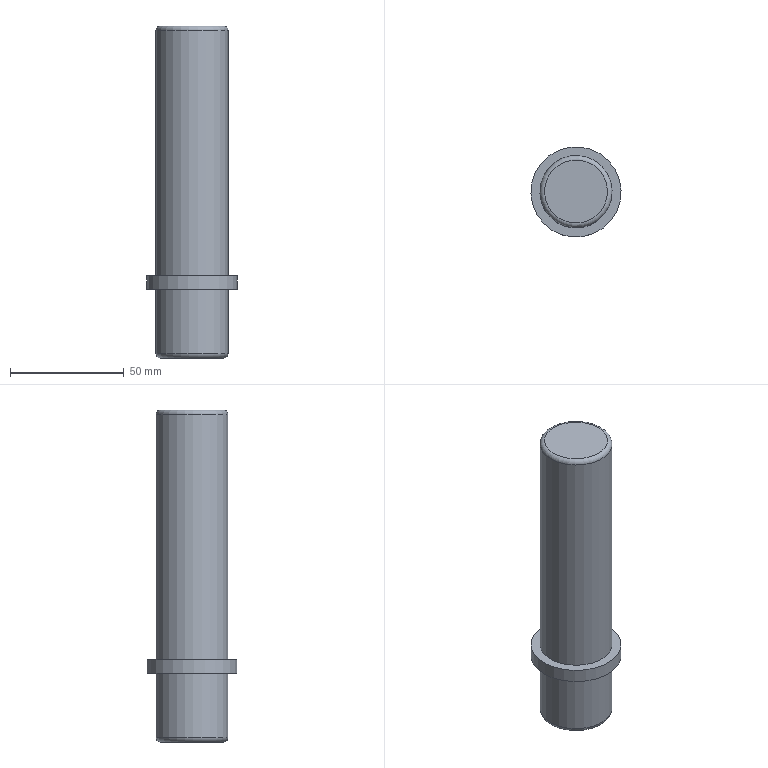Part | STEP file | 1_id1374_x_t | 1 solid | 13 faces | box 39.688 x 39.688 x 146.05 mm | volume 117725 mm3 | plane 5 | cylinder 4 | cone 2 | torus 2 | commonest cylinder face diameters 31.75 x2 4.2 x1 39.688 x1
STEP:
#1=CARTESIAN_POINT('',(0.,0.,0.));
#2=DIRECTION('',(0.,0.,1.));
#3=DIRECTION('',(1.,0.,0.));
#4=AXIS2_PLACEMENT_3D('',#1,#2,#3);
#5=CARTESIAN_POINT('',(862.606,287.316,48.075));
#6=VERTEX_POINT('',#5);
#7=CARTESIAN_POINT('',(862.925,287.5,48.075));
#8=DIRECTION('',(0.,0.,1.));
#9=DIRECTION('',(-0.866,-0.5,0.));
#10=AXIS2_PLACEMENT_3D('',#7,#8,#9);
#11=CIRCLE('',#10,0.3679);
#12=CARTESIAN_POINT('',(862.925,287.5,48.075));
#13=DIRECTION('',(0.,0.,1.));
#14=DIRECTION('',(-0.5,0.866,0.));
#15=AXIS2_PLACEMENT_3D('',#12,#13,#14);
#16=PLANE('',#15);
#17=CARTESIAN_POINT('',(0.0001996,0.));
#18=DIRECTION('',(0.,1.));
#19=AXIS2_PLACEMENT_2D('',#17,#18);
#20=CIRCLE('',#19,0.3679);
#21=(GEOMETRIC_REPRESENTATION_CONTEXT(2)PARAMETRIC_REPRESENTATION_CONTEXT()REPRESENTATION_CONTEXT('',''));
#22=DEFINITIONAL_REPRESENTATION('',(#20),#21);
#23=PCURVE('',#16,#22);
#24=CARTESIAN_POINT('',(862.925,287.5,47.575));
#25=DIRECTION('',(0.,0.,-1.));
#26=DIRECTION('',(-0.866,-0.5,0.));
#27=AXIS2_PLACEMENT_3D('',#24,#25,#26);
#28=CONICAL_SURFACE('',#27,1.234,1.047);
#29=CARTESIAN_POINT('',(6.283,-0.5));
#30=DIRECTION('',(-1.,0.));
#31=VECTOR('',#30,1.);
#32=LINE('',#29,#31);
#33=(GEOMETRIC_REPRESENTATION_CONTEXT(2)PARAMETRIC_REPRESENTATION_CONTEXT()REPRESENTATION_CONTEXT('',''));
#34=DEFINITIONAL_REPRESENTATION('',(#32),#33);
#35=PCURVE('',#28,#34);
#36=SURFACE_CURVE('',#11,(#23,#35),.PCURVE_S1.);
#37=EDGE_CURVE('',#6,#6,#36,.T.);
#38=ORIENTED_EDGE('',*,*,#37,.F.);
#39=EDGE_LOOP('',(#38));
#40=FACE_BOUND('',#39,.T.);
#41=ADVANCED_FACE('',(#40),#16,.F.);
#42=CARTESIAN_POINT('',(861.106,286.45,47.075));
#43=VERTEX_POINT('',#42);
#44=CARTESIAN_POINT('',(864.744,288.55,47.075));
#45=VERTEX_POINT('',#44);
#46=CARTESIAN_POINT('',(862.925,287.5,47.075));
#47=DIRECTION('',(0.,0.,-1.));
#48=DIRECTION('',(0.866,0.5,0.));
#49=AXIS2_PLACEMENT_3D('',#46,#47,#48);
#50=CIRCLE('',#49,2.1);
#51=CARTESIAN_POINT('',(-3.142,0.5));
#52=DIRECTION('',(1.,0.));
#53=VECTOR('',#52,1.);
#54=LINE('',#51,#53);
#55=(GEOMETRIC_REPRESENTATION_CONTEXT(2)PARAMETRIC_REPRESENTATION_CONTEXT()REPRESENTATION_CONTEXT('',''));
#56=DEFINITIONAL_REPRESENTATION('',(#54),#55);
#57=PCURVE('',#28,#56);
#58=CARTESIAN_POINT('',(862.925,287.5,47.075));
#59=DIRECTION('',(0.,0.,1.));
#60=DIRECTION('',(-0.866,-0.5,0.));
#61=AXIS2_PLACEMENT_3D('',#58,#59,#60);
#62=CYLINDRICAL_SURFACE('',#61,2.1);
#63=CARTESIAN_POINT('',(9.425,0.));
#64=DIRECTION('',(-1.,0.));
#65=VECTOR('',#64,1.);
#66=LINE('',#63,#65);
#67=(GEOMETRIC_REPRESENTATION_CONTEXT(2)PARAMETRIC_REPRESENTATION_CONTEXT()REPRESENTATION_CONTEXT('',''));
#68=DEFINITIONAL_REPRESENTATION('',(#66),#67);
#69=PCURVE('',#62,#68);
#70=SURFACE_CURVE('',#50,(#57,#69),.PCURVE_S1.);
#71=EDGE_CURVE('',#43,#45,#70,.T.);
#72=ORIENTED_EDGE('',*,*,#71,.F.);
#73=CARTESIAN_POINT('',(862.606,287.316,48.075));
#74=CARTESIAN_POINT('',(861.106,286.45,47.075));
#75=B_SPLINE_CURVE_WITH_KNOTS('',1,(#73,#74),.UNSPECIFIED.,.F.,.F.,(2,2),(-1.,1.),.PIECEWISE_BEZIER_KNOTS.);
#76=CARTESIAN_POINT('',(0.,0.));
#77=DIRECTION('',(0.,1.));
#78=VECTOR('',#77,1.);
#79=LINE('',#76,#78);
#80=(GEOMETRIC_REPRESENTATION_CONTEXT(2)PARAMETRIC_REPRESENTATION_CONTEXT()REPRESENTATION_CONTEXT('',''));
#81=DEFINITIONAL_REPRESENTATION('',(#79),#80);
#82=PCURVE('',#28,#81);
#83=CARTESIAN_POINT('',(6.283,0.));
#84=DIRECTION('',(0.,1.));
#85=VECTOR('',#84,1.);
#86=LINE('',#83,#85);
#87=(GEOMETRIC_REPRESENTATION_CONTEXT(2)PARAMETRIC_REPRESENTATION_CONTEXT()REPRESENTATION_CONTEXT('',''));
#88=DEFINITIONAL_REPRESENTATION('',(#86),#87);
#89=PCURVE('',#28,#88);
#90=SEAM_CURVE('',#75,(#82,#89),.PCURVE_S1.);
#91=EDGE_CURVE('',#6,#43,#90,.T.);
#92=ORIENTED_EDGE('',*,*,#91,.F.);
#93=ORIENTED_EDGE('',*,*,#37,.F.);
#94=ORIENTED_EDGE('',*,*,#91,.T.);
#95=CARTESIAN_POINT('',(862.925,287.5,47.075));
#96=DIRECTION('',(0.,0.,-1.));
#97=DIRECTION('',(0.866,0.5,0.));
#98=AXIS2_PLACEMENT_3D('',#95,#96,#97);
#99=CIRCLE('',#98,2.1);
#100=CARTESIAN_POINT('',(3.142,0.5));
#101=DIRECTION('',(1.,0.));
#102=VECTOR('',#101,1.);
#103=LINE('',#100,#102);
#104=(GEOMETRIC_REPRESENTATION_CONTEXT(2)PARAMETRIC_REPRESENTATION_CONTEXT()REPRESENTATION_CONTEXT('',''));
#105=DEFINITIONAL_REPRESENTATION('',(#103),#104);
#106=PCURVE('',#28,#105);
#107=CARTESIAN_POINT('',(9.425,0.));
#108=DIRECTION('',(-1.,0.));
#109=VECTOR('',#108,1.);
#110=LINE('',#107,#109);
#111=(GEOMETRIC_REPRESENTATION_CONTEXT(2)PARAMETRIC_REPRESENTATION_CONTEXT()REPRESENTATION_CONTEXT('',''));
#112=DEFINITIONAL_REPRESENTATION('',(#110),#111);
#113=PCURVE('',#62,#112);
#114=SURFACE_CURVE('',#99,(#106,#113),.PCURVE_S1.);
#115=EDGE_CURVE('',#45,#43,#114,.T.);
#116=ORIENTED_EDGE('',*,*,#115,.F.);
#117=EDGE_LOOP('',(#72,#92,#93,#94,#116));
#118=FACE_BOUND('',#117,.F.);
#119=ADVANCED_FACE('',(#118),#28,.F.);
#120=ORIENTED_EDGE('',*,*,#71,.T.);
#121=CARTESIAN_POINT('',(864.744,288.55,18.575));
#122=VERTEX_POINT('',#121);
#123=CARTESIAN_POINT('',(864.744,288.55,18.575));
#124=CARTESIAN_POINT('',(864.744,288.55,47.075));
#125=B_SPLINE_CURVE_WITH_KNOTS('',1,(#123,#124),.UNSPECIFIED.,.F.,.F.,(2,2),(-28.5,0.),.PIECEWISE_BEZIER_KNOTS.);
#126=CARTESIAN_POINT('',(3.142,0.));
#127=DIRECTION('',(0.,1.));
#128=VECTOR('',#127,1.);
#129=LINE('',#126,#128);
#130=(GEOMETRIC_REPRESENTATION_CONTEXT(2)PARAMETRIC_REPRESENTATION_CONTEXT()REPRESENTATION_CONTEXT('',''));
#131=DEFINITIONAL_REPRESENTATION('',(#129),#130);
#132=PCURVE('',#62,#131);
#133=CARTESIAN_POINT('',(9.425,0.));
#134=DIRECTION('',(0.,1.));
#135=VECTOR('',#134,1.);
#136=LINE('',#133,#135);
#137=(GEOMETRIC_REPRESENTATION_CONTEXT(2)PARAMETRIC_REPRESENTATION_CONTEXT()REPRESENTATION_CONTEXT('',''));
#138=DEFINITIONAL_REPRESENTATION('',(#136),#137);
#139=PCURVE('',#62,#138);
#140=SEAM_CURVE('',#125,(#132,#139),.PCURVE_S1.);
#141=EDGE_CURVE('',#122,#45,#140,.T.);
#142=ORIENTED_EDGE('',*,*,#141,.F.);
#143=CARTESIAN_POINT('',(861.106,286.45,18.575));
#144=VERTEX_POINT('',#143);
#145=CARTESIAN_POINT('',(862.925,287.5,18.575));
#146=DIRECTION('',(0.,0.,1.));
#147=DIRECTION('',(0.866,0.5,0.));
#148=AXIS2_PLACEMENT_3D('',#145,#146,#147);
#149=CIRCLE('',#148,2.1);
#150=CARTESIAN_POINT('',(3.142,-28.5));
#151=DIRECTION('',(1.,0.));
#152=VECTOR('',#151,1.);
#153=LINE('',#150,#152);
#154=(GEOMETRIC_REPRESENTATION_CONTEXT(2)PARAMETRIC_REPRESENTATION_CONTEXT()REPRESENTATION_CONTEXT('',''));
#155=DEFINITIONAL_REPRESENTATION('',(#153),#154);
#156=PCURVE('',#62,#155);
#157=CARTESIAN_POINT('',(862.925,287.5,18.244));
#158=DIRECTION('',(0.,0.,-1.));
#159=DIRECTION('',(-0.866,-0.5,0.));
#160=AXIS2_PLACEMENT_3D('',#157,#158,#159);
#161=CONICAL_SURFACE('',#160,2.431,0.7854);
#162=CARTESIAN_POINT('',(3.142,-0.3313));
#163=DIRECTION('',(-1.,0.));
#164=VECTOR('',#163,1.);
#165=LINE('',#162,#164);
#166=(GEOMETRIC_REPRESENTATION_CONTEXT(2)PARAMETRIC_REPRESENTATION_CONTEXT()REPRESENTATION_CONTEXT('',''));
#167=DEFINITIONAL_REPRESENTATION('',(#165),#166);
#168=PCURVE('',#161,#167);
#169=SURFACE_CURVE('',#149,(#156,#168),.PCURVE_S1.);
#170=EDGE_CURVE('',#122,#144,#169,.T.);
#171=ORIENTED_EDGE('',*,*,#170,.T.);
#172=CARTESIAN_POINT('',(862.925,287.5,18.575));
#173=DIRECTION('',(0.,0.,1.));
#174=DIRECTION('',(0.866,0.5,0.));
#175=AXIS2_PLACEMENT_3D('',#172,#173,#174);
#176=CIRCLE('',#175,2.1);
#177=CARTESIAN_POINT('',(3.142,-28.5));
#178=DIRECTION('',(1.,0.));
#179=VECTOR('',#178,1.);
#180=LINE('',#177,#179);
#181=(GEOMETRIC_REPRESENTATION_CONTEXT(2)PARAMETRIC_REPRESENTATION_CONTEXT()REPRESENTATION_CONTEXT('',''));
#182=DEFINITIONAL_REPRESENTATION('',(#180),#181);
#183=PCURVE('',#62,#182);
#184=CARTESIAN_POINT('',(9.425,-0.3313));
#185=DIRECTION('',(-1.,0.));
#186=VECTOR('',#185,1.);
#187=LINE('',#184,#186);
#188=(GEOMETRIC_REPRESENTATION_CONTEXT(2)PARAMETRIC_REPRESENTATION_CONTEXT()REPRESENTATION_CONTEXT('',''));
#189=DEFINITIONAL_REPRESENTATION('',(#187),#188);
#190=PCURVE('',#161,#189);
#191=SURFACE_CURVE('',#176,(#183,#190),.PCURVE_S1.);
#192=EDGE_CURVE('',#144,#122,#191,.T.);
#193=ORIENTED_EDGE('',*,*,#192,.T.);
#194=ORIENTED_EDGE('',*,*,#141,.T.);
#195=ORIENTED_EDGE('',*,*,#115,.T.);
#196=EDGE_LOOP('',(#120,#142,#171,#193,#194,#195));
#197=FACE_BOUND('',#196,.F.);
#198=ADVANCED_FACE('',(#197),#62,.F.);
#199=CARTESIAN_POINT('',(860.533,286.119,17.912));
#200=VERTEX_POINT('',#199);
#201=CARTESIAN_POINT('',(862.925,287.5,17.912));
#202=DIRECTION('',(0.,0.,1.));
#203=DIRECTION('',(-0.866,-0.5,0.));
#204=AXIS2_PLACEMENT_3D('',#201,#202,#203);
#205=CIRCLE('',#204,2.763);
#206=CARTESIAN_POINT('',(6.283,0.3313));
#207=DIRECTION('',(-1.,0.));
#208=VECTOR('',#207,1.);
#209=LINE('',#206,#208);
#210=(GEOMETRIC_REPRESENTATION_CONTEXT(2)PARAMETRIC_REPRESENTATION_CONTEXT()REPRESENTATION_CONTEXT('',''));
#211=DEFINITIONAL_REPRESENTATION('',(#209),#210);
#212=PCURVE('',#161,#211);
#213=CARTESIAN_POINT('',(862.925,287.5,17.912));
#214=DIRECTION('',(0.,0.,1.));
#215=DIRECTION('',(-0.866,-0.5,0.));
#216=AXIS2_PLACEMENT_3D('',#213,#214,#215);
#217=PLANE('',#216);
#218=CARTESIAN_POINT('',(0.,0.));
#219=DIRECTION('',(1.,0.));
#220=AXIS2_PLACEMENT_2D('',#218,#219);
#221=CIRCLE('',#220,2.763);
#222=(GEOMETRIC_REPRESENTATION_CONTEXT(2)PARAMETRIC_REPRESENTATION_CONTEXT()REPRESENTATION_CONTEXT('',''));
#223=DEFINITIONAL_REPRESENTATION('',(#221),#222);
#224=PCURVE('',#217,#223);
#225=SURFACE_CURVE('',#205,(#212,#224),.PCURVE_S1.);
#226=EDGE_CURVE('',#200,#200,#225,.T.);
#227=ORIENTED_EDGE('',*,*,#226,.T.);
#228=CARTESIAN_POINT('',(861.106,286.45,18.575));
#229=CARTESIAN_POINT('',(860.533,286.119,17.912));
#230=B_SPLINE_CURVE_WITH_KNOTS('',1,(#228,#229),.UNSPECIFIED.,.F.,.F.,(2,2),(-0.4685,0.4685),.PIECEWISE_BEZIER_KNOTS.);
#231=CARTESIAN_POINT('',(0.,0.));
#232=DIRECTION('',(0.,1.));
#233=VECTOR('',#232,1.);
#234=LINE('',#231,#233);
#235=(GEOMETRIC_REPRESENTATION_CONTEXT(2)PARAMETRIC_REPRESENTATION_CONTEXT()REPRESENTATION_CONTEXT('',''));
#236=DEFINITIONAL_REPRESENTATION('',(#234),#235);
#237=PCURVE('',#161,#236);
#238=CARTESIAN_POINT('',(6.283,0.));
#239=DIRECTION('',(0.,1.));
#240=VECTOR('',#239,1.);
#241=LINE('',#238,#240);
#242=(GEOMETRIC_REPRESENTATION_CONTEXT(2)PARAMETRIC_REPRESENTATION_CONTEXT()REPRESENTATION_CONTEXT('',''));
#243=DEFINITIONAL_REPRESENTATION('',(#241),#242);
#244=PCURVE('',#161,#243);
#245=SEAM_CURVE('',#230,(#237,#244),.PCURVE_S1.);
#246=EDGE_CURVE('',#144,#200,#245,.T.);
#247=ORIENTED_EDGE('',*,*,#246,.F.);
#248=ORIENTED_EDGE('',*,*,#170,.F.);
#249=ORIENTED_EDGE('',*,*,#192,.F.);
#250=ORIENTED_EDGE('',*,*,#246,.T.);
#251=EDGE_LOOP('',(#227,#247,#248,#249,#250));
#252=FACE_BOUND('',#251,.F.);
#253=ADVANCED_FACE('',(#252),#161,.F.);
#254=CARTESIAN_POINT('',(874.941,294.438,17.912));
#255=VERTEX_POINT('',#254);
#256=CARTESIAN_POINT('',(850.909,280.562,17.912));
#257=VERTEX_POINT('',#256);
#258=CARTESIAN_POINT('',(862.925,287.5,17.912));
#259=DIRECTION('',(0.,0.,-1.));
#260=DIRECTION('',(0.866,0.5,0.));
#261=AXIS2_PLACEMENT_3D('',#258,#259,#260);
#262=CIRCLE('',#261,13.875);
#263=CARTESIAN_POINT('',(-13.875,0.));
#264=CARTESIAN_POINT('',(-13.875,24.032));
#265=CARTESIAN_POINT('',(6.938,12.016));
#266=CARTESIAN_POINT('',(27.75,0.));
#267=CARTESIAN_POINT('',(6.938,-12.016));
#268=CARTESIAN_POINT('',(-13.875,-24.032));
#269=CARTESIAN_POINT('',(-13.875,0.));
#270=(BOUNDED_CURVE()B_SPLINE_CURVE(2,(#263,#264,#265,#266,#267,#268,#269),.UNSPECIFIED.,.T.,.F.)B_SPLINE_CURVE_WITH_KNOTS((1,2,2,2,2,1),(-2.094,0.,2.094,4.189,6.283,8.378),.UNSPECIFIED.)CURVE()GEOMETRIC_REPRESENTATION_ITEM()RATIONAL_B_SPLINE_CURVE((1.,0.5,1.,0.5,1.,0.5,1.))REPRESENTATION_ITEM(''));
#271=(GEOMETRIC_REPRESENTATION_CONTEXT(2)PARAMETRIC_REPRESENTATION_CONTEXT()REPRESENTATION_CONTEXT('',''));
#272=DEFINITIONAL_REPRESENTATION('',(#270),#271);
#273=PCURVE('',#217,#272);
#274=CARTESIAN_POINT('',(862.925,287.5,19.912));
#275=DIRECTION('',(0.,0.,1.));
#276=DIRECTION('',(-0.866,-0.5,0.));
#277=AXIS2_PLACEMENT_3D('',#274,#275,#276);
#278=TOROIDAL_SURFACE('',#277,13.875,2.);
#279=CARTESIAN_POINT('',(3.142,4.712));
#280=DIRECTION('',(-1.,0.));
#281=VECTOR('',#280,1.);
#282=LINE('',#279,#281);
#283=(GEOMETRIC_REPRESENTATION_CONTEXT(2)PARAMETRIC_REPRESENTATION_CONTEXT()REPRESENTATION_CONTEXT('',''));
#284=DEFINITIONAL_REPRESENTATION('',(#282),#283);
#285=PCURVE('',#278,#284);
#286=SURFACE_CURVE('',#262,(#273,#285),.PCURVE_S1.);
#287=EDGE_CURVE('',#255,#257,#286,.T.);
#288=ORIENTED_EDGE('',*,*,#287,.T.);
#289=CARTESIAN_POINT('',(862.925,287.5,17.912));
#290=DIRECTION('',(0.,0.,-1.));
#291=DIRECTION('',(0.866,0.5,0.));
#292=AXIS2_PLACEMENT_3D('',#289,#290,#291);
#293=CIRCLE('',#292,13.875);
#294=CARTESIAN_POINT('',(-13.875,0.));
#295=CARTESIAN_POINT('',(-13.875,24.032));
#296=CARTESIAN_POINT('',(6.938,12.016));
#297=CARTESIAN_POINT('',(27.75,0.));
#298=CARTESIAN_POINT('',(6.938,-12.016));
#299=CARTESIAN_POINT('',(-13.875,-24.032));
#300=CARTESIAN_POINT('',(-13.875,0.));
#301=(BOUNDED_CURVE()B_SPLINE_CURVE(2,(#294,#295,#296,#297,#298,#299,#300),.UNSPECIFIED.,.T.,.F.)B_SPLINE_CURVE_WITH_KNOTS((1,2,2,2,2,1),(-2.094,0.,2.094,4.189,6.283,8.378),.UNSPECIFIED.)CURVE()GEOMETRIC_REPRESENTATION_ITEM()RATIONAL_B_SPLINE_CURVE((1.,0.5,1.,0.5,1.,0.5,1.))REPRESENTATION_ITEM(''));
#302=(GEOMETRIC_REPRESENTATION_CONTEXT(2)PARAMETRIC_REPRESENTATION_CONTEXT()REPRESENTATION_CONTEXT('',''));
#303=DEFINITIONAL_REPRESENTATION('',(#301),#302);
#304=PCURVE('',#217,#303);
#305=CARTESIAN_POINT('',(9.425,4.712));
#306=DIRECTION('',(-1.,0.));
#307=VECTOR('',#306,1.);
#308=LINE('',#305,#307);
#309=(GEOMETRIC_REPRESENTATION_CONTEXT(2)PARAMETRIC_REPRESENTATION_CONTEXT()REPRESENTATION_CONTEXT('',''));
#310=DEFINITIONAL_REPRESENTATION('',(#308),#309);
#311=PCURVE('',#278,#310);
#312=SURFACE_CURVE('',#293,(#304,#311),.PCURVE_S1.);
#313=EDGE_CURVE('',#257,#255,#312,.T.);
#314=ORIENTED_EDGE('',*,*,#313,.T.);
#315=EDGE_LOOP('',(#288,#314));
#316=FACE_BOUND('',#315,.T.);
#317=ORIENTED_EDGE('',*,*,#226,.T.);
#318=EDGE_LOOP('',(#317));
#319=FACE_BOUND('',#318,.T.);
#320=ADVANCED_FACE('',(#316,#319),#217,.F.);
#321=CARTESIAN_POINT('',(849.177,279.562,19.912));
#322=VERTEX_POINT('',#321);
#323=CARTESIAN_POINT('',(876.673,295.438,19.912));
#324=VERTEX_POINT('',#323);
#325=CARTESIAN_POINT('',(862.925,287.5,19.912));
#326=DIRECTION('',(0.,0.,-1.));
#327=DIRECTION('',(-0.866,-0.5,0.));
#328=AXIS2_PLACEMENT_3D('',#325,#326,#327);
#329=CIRCLE('',#328,15.875);
#330=CARTESIAN_POINT('',(6.283,6.283));
#331=DIRECTION('',(-1.,0.));
#332=VECTOR('',#331,1.);
#333=LINE('',#330,#332);
#334=(GEOMETRIC_REPRESENTATION_CONTEXT(2)PARAMETRIC_REPRESENTATION_CONTEXT()REPRESENTATION_CONTEXT('',''));
#335=DEFINITIONAL_REPRESENTATION('',(#333),#334);
#336=PCURVE('',#278,#335);
#337=CARTESIAN_POINT('',(862.925,287.5,18.075));
#338=DIRECTION('',(0.,0.,-1.));
#339=DIRECTION('',(0.866,0.5,0.));
#340=AXIS2_PLACEMENT_3D('',#337,#338,#339);
#341=CYLINDRICAL_SURFACE('',#340,15.875);
#342=CARTESIAN_POINT('',(3.142,-1.837));
#343=DIRECTION('',(1.,0.));
#344=VECTOR('',#343,1.);
#345=LINE('',#342,#344);
#346=(GEOMETRIC_REPRESENTATION_CONTEXT(2)PARAMETRIC_REPRESENTATION_CONTEXT()REPRESENTATION_CONTEXT('',''));
#347=DEFINITIONAL_REPRESENTATION('',(#345),#346);
#348=PCURVE('',#341,#347);
#349=SURFACE_CURVE('',#329,(#336,#348),.PCURVE_S1.);
#350=EDGE_CURVE('',#322,#324,#349,.T.);
#351=ORIENTED_EDGE('',*,*,#350,.T.);
#352=CARTESIAN_POINT('',(862.925,287.5,19.912));
#353=DIRECTION('',(0.,0.,-1.));
#354=DIRECTION('',(-0.866,-0.5,0.));
#355=AXIS2_PLACEMENT_3D('',#352,#353,#354);
#356=CIRCLE('',#355,15.875);
#357=CARTESIAN_POINT('',(6.283,6.283));
#358=DIRECTION('',(-1.,0.));
#359=VECTOR('',#358,1.);
#360=LINE('',#357,#359);
#361=(GEOMETRIC_REPRESENTATION_CONTEXT(2)PARAMETRIC_REPRESENTATION_CONTEXT()REPRESENTATION_CONTEXT('',''));
#362=DEFINITIONAL_REPRESENTATION('',(#360),#361);
#363=PCURVE('',#278,#362);
#364=CARTESIAN_POINT('',(-3.142,-1.837));
#365=DIRECTION('',(1.,0.));
#366=VECTOR('',#365,1.);
#367=LINE('',#364,#366);
#368=(GEOMETRIC_REPRESENTATION_CONTEXT(2)PARAMETRIC_REPRESENTATION_CONTEXT()REPRESENTATION_CONTEXT('',''));
#369=DEFINITIONAL_REPRESENTATION('',(#367),#368);
#370=PCURVE('',#341,#369);
#371=SURFACE_CURVE('',#356,(#363,#370),.PCURVE_S1.);
#372=EDGE_CURVE('',#324,#322,#371,.T.);
#373=ORIENTED_EDGE('',*,*,#372,.T.);
#374=CARTESIAN_POINT('',(850.909,280.562,17.912));
#375=CARTESIAN_POINT('',(850.446,280.295,17.912));
#376=CARTESIAN_POINT('',(849.995,280.035,18.083));
#377=CARTESIAN_POINT('',(849.607,279.811,18.409));
#378=CARTESIAN_POINT('',(849.324,279.648,18.857));
#379=CARTESIAN_POINT('',(849.177,279.562,19.378));
#380=CARTESIAN_POINT('',(849.177,279.562,19.912));
#381=(BOUNDED_CURVE()B_SPLINE_CURVE(6,(#374,#375,#376,#377,#378,#379,#380),.UNSPECIFIED.,.F.,.F.)B_SPLINE_CURVE_WITH_KNOTS((7,7),(-1.571,0.),.PIECEWISE_BEZIER_KNOTS.)CURVE()GEOMETRIC_REPRESENTATION_ITEM()RATIONAL_B_SPLINE_CURVE((1.031,1.01,0.9979,0.994,0.9979,1.01,1.031))REPRESENTATION_ITEM(''));
#382=CARTESIAN_POINT('',(0.,6.283));
#383=DIRECTION('',(0.,1.));
#384=VECTOR('',#383,1.);
#385=LINE('',#382,#384);
#386=(GEOMETRIC_REPRESENTATION_CONTEXT(2)PARAMETRIC_REPRESENTATION_CONTEXT()REPRESENTATION_CONTEXT('',''));
#387=DEFINITIONAL_REPRESENTATION('',(#385),#386);
#388=PCURVE('',#278,#387);
#389=CARTESIAN_POINT('',(6.283,6.283));
#390=DIRECTION('',(0.,1.));
#391=VECTOR('',#390,1.);
#392=LINE('',#389,#391);
#393=(GEOMETRIC_REPRESENTATION_CONTEXT(2)PARAMETRIC_REPRESENTATION_CONTEXT()REPRESENTATION_CONTEXT('',''));
#394=DEFINITIONAL_REPRESENTATION('',(#392),#393);
#395=PCURVE('',#278,#394);
#396=SEAM_CURVE('',#381,(#388,#395),.PCURVE_S1.);
#397=EDGE_CURVE('',#257,#322,#396,.T.);
#398=ORIENTED_EDGE('',*,*,#397,.F.);
#399=ORIENTED_EDGE('',*,*,#287,.F.);
#400=ORIENTED_EDGE('',*,*,#313,.F.);
#401=ORIENTED_EDGE('',*,*,#397,.T.);
#402=EDGE_LOOP('',(#351,#373,#398,#399,#400,#401));
#403=FACE_BOUND('',#402,.T.);
#404=ADVANCED_FACE('',(#403),#278,.T.);
#405=ORIENTED_EDGE('',*,*,#372,.F.);
#406=CARTESIAN_POINT('',(876.673,295.438,48.075));
#407=VERTEX_POINT('',#406);
#408=CARTESIAN_POINT('',(876.673,295.438,48.075));
#409=CARTESIAN_POINT('',(876.673,295.438,19.912));
#410=B_SPLINE_CURVE_WITH_KNOTS('',1,(#408,#409),.UNSPECIFIED.,.F.,.F.,(2,2),(-30.,-1.837),.PIECEWISE_BEZIER_KNOTS.);
#411=CARTESIAN_POINT('',(0.,0.));
#412=DIRECTION('',(0.,1.));
#413=VECTOR('',#412,1.);
#414=LINE('',#411,#413);
#415=(GEOMETRIC_REPRESENTATION_CONTEXT(2)PARAMETRIC_REPRESENTATION_CONTEXT()REPRESENTATION_CONTEXT('',''));
#416=DEFINITIONAL_REPRESENTATION('',(#414),#415);
#417=PCURVE('',#341,#416);
#418=CARTESIAN_POINT('',(6.283,0.));
#419=DIRECTION('',(0.,1.));
#420=VECTOR('',#419,1.);
#421=LINE('',#418,#420);
#422=(GEOMETRIC_REPRESENTATION_CONTEXT(2)PARAMETRIC_REPRESENTATION_CONTEXT()REPRESENTATION_CONTEXT('',''));
#423=DEFINITIONAL_REPRESENTATION('',(#421),#422);
#424=PCURVE('',#341,#423);
#425=SEAM_CURVE('',#410,(#417,#424),.PCURVE_S1.);
#426=EDGE_CURVE('',#407,#324,#425,.T.);
#427=ORIENTED_EDGE('',*,*,#426,.F.);
#428=CARTESIAN_POINT('',(862.925,287.5,48.075));
#429=DIRECTION('',(0.,0.,1.));
#430=DIRECTION('',(0.866,0.5,0.));
#431=AXIS2_PLACEMENT_3D('',#428,#429,#430);
#432=CIRCLE('',#431,15.875);
#433=CARTESIAN_POINT('',(6.283,-30.));
#434=DIRECTION('',(-1.,0.));
#435=VECTOR('',#434,1.);
#436=LINE('',#433,#435);
#437=(GEOMETRIC_REPRESENTATION_CONTEXT(2)PARAMETRIC_REPRESENTATION_CONTEXT()REPRESENTATION_CONTEXT('',''));
#438=DEFINITIONAL_REPRESENTATION('',(#436),#437);
#439=PCURVE('',#341,#438);
#440=CARTESIAN_POINT('',(862.925,287.5,48.075));
#441=DIRECTION('',(0.,0.,1.));
#442=DIRECTION('',(-0.5,0.866,0.));
#443=AXIS2_PLACEMENT_3D('',#440,#441,#442);
#444=PLANE('',#443);
#445=CARTESIAN_POINT('',(0.000000444,-0.000000024));
#446=DIRECTION('',(0.,-1.));
#447=AXIS2_PLACEMENT_2D('',#445,#446);
#448=CIRCLE('',#447,15.875);
#449=(GEOMETRIC_REPRESENTATION_CONTEXT(2)PARAMETRIC_REPRESENTATION_CONTEXT()REPRESENTATION_CONTEXT('',''));
#450=DEFINITIONAL_REPRESENTATION('',(#448),#449);
#451=PCURVE('',#444,#450);
#452=SURFACE_CURVE('',#432,(#439,#451),.PCURVE_S1.);
#453=EDGE_CURVE('',#407,#407,#452,.T.);
#454=ORIENTED_EDGE('',*,*,#453,.F.);
#455=ORIENTED_EDGE('',*,*,#426,.T.);
#456=ORIENTED_EDGE('',*,*,#350,.F.);
#457=EDGE_LOOP('',(#405,#427,#454,#455,#456));
#458=FACE_BOUND('',#457,.T.);
#459=ADVANCED_FACE('',(#458),#341,.T.);
#460=CARTESIAN_POINT('',(845.74,277.578,48.075));
#461=VERTEX_POINT('',#460);
#462=CARTESIAN_POINT('',(862.925,287.5,48.075));
#463=DIRECTION('',(0.,0.,-1.));
#464=DIRECTION('',(-0.866,-0.5,0.));
#465=AXIS2_PLACEMENT_3D('',#462,#463,#464);
#466=CIRCLE('',#465,19.844);
#467=CARTESIAN_POINT('',(0.000000444,19.844));
#468=CARTESIAN_POINT('',(34.37,19.844));
#469=CARTESIAN_POINT('',(17.185,-9.922));
#470=CARTESIAN_POINT('',(0.000000444,-39.688));
#471=CARTESIAN_POINT('',(-17.185,-9.922));
#472=CARTESIAN_POINT('',(-34.37,19.844));
#473=CARTESIAN_POINT('',(0.000000444,19.844));
#474=(BOUNDED_CURVE()B_SPLINE_CURVE(2,(#467,#468,#469,#470,#471,#472,#473),.UNSPECIFIED.,.T.,.F.)B_SPLINE_CURVE_WITH_KNOTS((1,2,2,2,2,1),(-2.094,0.,2.094,4.189,6.283,8.378),.UNSPECIFIED.)CURVE()GEOMETRIC_REPRESENTATION_ITEM()RATIONAL_B_SPLINE_CURVE((1.,0.5,1.,0.5,1.,0.5,1.))REPRESENTATION_ITEM(''));
#475=(GEOMETRIC_REPRESENTATION_CONTEXT(2)PARAMETRIC_REPRESENTATION_CONTEXT()REPRESENTATION_CONTEXT('',''));
#476=DEFINITIONAL_REPRESENTATION('',(#474),#475);
#477=PCURVE('',#444,#476);
#478=CARTESIAN_POINT('',(862.925,287.5,54.075));
#479=DIRECTION('',(0.,0.,1.));
#480=DIRECTION('',(-0.866,-0.5,0.));
#481=AXIS2_PLACEMENT_3D('',#478,#479,#480);
#482=CYLINDRICAL_SURFACE('',#481,19.844);
#483=CARTESIAN_POINT('',(6.283,-6.));
#484=DIRECTION('',(-1.,0.));
#485=VECTOR('',#484,1.);
#486=LINE('',#483,#485);
#487=(GEOMETRIC_REPRESENTATION_CONTEXT(2)PARAMETRIC_REPRESENTATION_CONTEXT()REPRESENTATION_CONTEXT('',''));
#488=DEFINITIONAL_REPRESENTATION('',(#486),#487);
#489=PCURVE('',#482,#488);
#490=SURFACE_CURVE('',#466,(#477,#489),.PCURVE_S1.);
#491=EDGE_CURVE('',#461,#461,#490,.T.);
#492=ORIENTED_EDGE('',*,*,#491,.T.);
#493=EDGE_LOOP('',(#492));
#494=FACE_BOUND('',#493,.T.);
#495=ORIENTED_EDGE('',*,*,#453,.T.);
#496=EDGE_LOOP('',(#495));
#497=FACE_BOUND('',#496,.T.);
#498=ADVANCED_FACE('',(#494,#497),#444,.F.);
#499=CARTESIAN_POINT('',(845.74,277.578,54.075));
#500=VERTEX_POINT('',#499);
#501=CARTESIAN_POINT('',(880.11,297.422,54.075));
#502=VERTEX_POINT('',#501);
#503=CARTESIAN_POINT('',(862.925,287.5,54.075));
#504=DIRECTION('',(0.,0.,1.));
#505=DIRECTION('',(0.866,0.5,0.));
#506=AXIS2_PLACEMENT_3D('',#503,#504,#505);
#507=CIRCLE('',#506,19.844);
#508=CARTESIAN_POINT('',(-3.142,0.));
#509=DIRECTION('',(1.,0.));
#510=VECTOR('',#509,1.);
#511=LINE('',#508,#510);
#512=(GEOMETRIC_REPRESENTATION_CONTEXT(2)PARAMETRIC_REPRESENTATION_CONTEXT()REPRESENTATION_CONTEXT('',''));
#513=DEFINITIONAL_REPRESENTATION('',(#511),#512);
#514=PCURVE('',#482,#513);
#515=CARTESIAN_POINT('',(862.925,287.5,54.075));
#516=DIRECTION('',(0.,0.,1.));
#517=DIRECTION('',(-0.866,-0.5,0.));
#518=AXIS2_PLACEMENT_3D('',#515,#516,#517);
#519=PLANE('',#518);
#520=CARTESIAN_POINT('',(0.,0.));
#521=DIRECTION('',(-1.,0.));
#522=AXIS2_PLACEMENT_2D('',#520,#521);
#523=CIRCLE('',#522,19.844);
#524=(GEOMETRIC_REPRESENTATION_CONTEXT(2)PARAMETRIC_REPRESENTATION_CONTEXT()REPRESENTATION_CONTEXT('',''));
#525=DEFINITIONAL_REPRESENTATION('',(#523),#524);
#526=PCURVE('',#519,#525);
#527=SURFACE_CURVE('',#507,(#514,#526),.PCURVE_S1.);
#528=EDGE_CURVE('',#500,#502,#527,.T.);
#529=ORIENTED_EDGE('',*,*,#528,.F.);
#530=CARTESIAN_POINT('',(845.74,277.578,48.075));
#531=CARTESIAN_POINT('',(845.74,277.578,54.075));
#532=B_SPLINE_CURVE_WITH_KNOTS('',1,(#530,#531),.UNSPECIFIED.,.F.,.F.,(2,2),(-6.,0.),.PIECEWISE_BEZIER_KNOTS.);
#533=CARTESIAN_POINT('',(0.,0.));
#534=DIRECTION('',(0.,1.));
#535=VECTOR('',#534,1.);
#536=LINE('',#533,#535);
#537=(GEOMETRIC_REPRESENTATION_CONTEXT(2)PARAMETRIC_REPRESENTATION_CONTEXT()REPRESENTATION_CONTEXT('',''));
#538=DEFINITIONAL_REPRESENTATION('',(#536),#537);
#539=PCURVE('',#482,#538);
#540=CARTESIAN_POINT('',(6.283,0.));
#541=DIRECTION('',(0.,1.));
#542=VECTOR('',#541,1.);
#543=LINE('',#540,#542);
#544=(GEOMETRIC_REPRESENTATION_CONTEXT(2)PARAMETRIC_REPRESENTATION_CONTEXT()REPRESENTATION_CONTEXT('',''));
#545=DEFINITIONAL_REPRESENTATION('',(#543),#544);
#546=PCURVE('',#482,#545);
#547=SEAM_CURVE('',#532,(#539,#546),.PCURVE_S1.);
#548=EDGE_CURVE('',#461,#500,#547,.T.);
#549=ORIENTED_EDGE('',*,*,#548,.F.);
#550=ORIENTED_EDGE('',*,*,#491,.F.);
#551=ORIENTED_EDGE('',*,*,#548,.T.);
#552=CARTESIAN_POINT('',(862.925,287.5,54.075));
#553=DIRECTION('',(0.,0.,1.));
#554=DIRECTION('',(0.866,0.5,0.));
#555=AXIS2_PLACEMENT_3D('',#552,#553,#554);
#556=CIRCLE('',#555,19.844);
#557=CARTESIAN_POINT('',(3.142,0.));
#558=DIRECTION('',(1.,0.));
#559=VECTOR('',#558,1.);
#560=LINE('',#557,#559);
#561=(GEOMETRIC_REPRESENTATION_CONTEXT(2)PARAMETRIC_REPRESENTATION_CONTEXT()REPRESENTATION_CONTEXT('',''));
#562=DEFINITIONAL_REPRESENTATION('',(#560),#561);
#563=PCURVE('',#482,#562);
#564=CARTESIAN_POINT('',(0.,0.));
#565=DIRECTION('',(-1.,0.));
#566=AXIS2_PLACEMENT_2D('',#564,#565);
#567=CIRCLE('',#566,19.844);
#568=(GEOMETRIC_REPRESENTATION_CONTEXT(2)PARAMETRIC_REPRESENTATION_CONTEXT()REPRESENTATION_CONTEXT('',''));
#569=DEFINITIONAL_REPRESENTATION('',(#567),#568);
#570=PCURVE('',#519,#569);
#571=SURFACE_CURVE('',#556,(#563,#570),.PCURVE_S1.);
#572=EDGE_CURVE('',#502,#500,#571,.T.);
#573=ORIENTED_EDGE('',*,*,#572,.F.);
#574=EDGE_LOOP('',(#529,#549,#550,#551,#573));
#575=FACE_BOUND('',#574,.T.);
#576=ADVANCED_FACE('',(#575),#482,.T.);
#577=ORIENTED_EDGE('',*,*,#572,.T.);
#578=ORIENTED_EDGE('',*,*,#528,.T.);
#579=EDGE_LOOP('',(#577,#578));
#580=FACE_BOUND('',#579,.T.);
#581=CARTESIAN_POINT('',(849.177,279.562,54.075));
#582=VERTEX_POINT('',#581);
#583=CARTESIAN_POINT('',(862.925,287.5,54.075));
#584=DIRECTION('',(0.,0.,-1.));
#585=DIRECTION('',(-0.866,-0.5,0.));
#586=AXIS2_PLACEMENT_3D('',#583,#584,#585);
#587=CIRCLE('',#586,15.875);
#588=CARTESIAN_POINT('',(15.875,0.));
#589=CARTESIAN_POINT('',(15.875,-27.496));
#590=CARTESIAN_POINT('',(-7.938,-13.748));
#591=CARTESIAN_POINT('',(-31.75,0.));
#592=CARTESIAN_POINT('',(-7.938,13.748));
#593=CARTESIAN_POINT('',(15.875,27.496));
#594=CARTESIAN_POINT('',(15.875,0.));
#595=(BOUNDED_CURVE()B_SPLINE_CURVE(2,(#588,#589,#590,#591,#592,#593,#594),.UNSPECIFIED.,.T.,.F.)B_SPLINE_CURVE_WITH_KNOTS((1,2,2,2,2,1),(-2.094,0.,2.094,4.189,6.283,8.378),.UNSPECIFIED.)CURVE()GEOMETRIC_REPRESENTATION_ITEM()RATIONAL_B_SPLINE_CURVE((1.,0.5,1.,0.5,1.,0.5,1.))REPRESENTATION_ITEM(''));
#596=(GEOMETRIC_REPRESENTATION_CONTEXT(2)PARAMETRIC_REPRESENTATION_CONTEXT()REPRESENTATION_CONTEXT('',''));
#597=DEFINITIONAL_REPRESENTATION('',(#595),#596);
#598=PCURVE('',#519,#597);
#599=CARTESIAN_POINT('',(862.925,287.5,139.025));
#600=DIRECTION('',(0.,0.,1.));
#601=DIRECTION('',(-0.866,-0.5,0.));
#602=AXIS2_PLACEMENT_3D('',#599,#600,#601);
#603=CYLINDRICAL_SURFACE('',#602,15.875);
#604=CARTESIAN_POINT('',(6.283,-84.95));
#605=DIRECTION('',(-1.,0.));
#606=VECTOR('',#605,1.);
#607=LINE('',#604,#606);
#608=(GEOMETRIC_REPRESENTATION_CONTEXT(2)PARAMETRIC_REPRESENTATION_CONTEXT()REPRESENTATION_CONTEXT('',''));
#609=DEFINITIONAL_REPRESENTATION('',(#607),#608);
#610=PCURVE('',#603,#609);
#611=SURFACE_CURVE('',#587,(#598,#610),.PCURVE_S1.);
#612=EDGE_CURVE('',#582,#582,#611,.T.);
#613=ORIENTED_EDGE('',*,*,#612,.T.);
#614=EDGE_LOOP('',(#613));
#615=FACE_BOUND('',#614,.T.);
#616=ADVANCED_FACE('',(#580,#615),#519,.T.);
#617=CARTESIAN_POINT('',(849.177,279.562,161.962));
#618=VERTEX_POINT('',#617);
#619=CARTESIAN_POINT('',(876.673,295.438,161.962));
#620=VERTEX_POINT('',#619);
#621=CARTESIAN_POINT('',(862.925,287.5,161.962));
#622=DIRECTION('',(0.,0.,1.));
#623=DIRECTION('',(0.866,0.5,0.));
#624=AXIS2_PLACEMENT_3D('',#621,#622,#623);
#625=CIRCLE('',#624,15.875);
#626=CARTESIAN_POINT('',(-3.142,22.938));
#627=DIRECTION('',(1.,0.));
#628=VECTOR('',#627,1.);
#629=LINE('',#626,#628);
#630=(GEOMETRIC_REPRESENTATION_CONTEXT(2)PARAMETRIC_REPRESENTATION_CONTEXT()REPRESENTATION_CONTEXT('',''));
#631=DEFINITIONAL_REPRESENTATION('',(#629),#630);
#632=PCURVE('',#603,#631);
#633=CARTESIAN_POINT('',(862.925,287.5,161.962));
#634=DIRECTION('',(0.,0.,1.));
#635=DIRECTION('',(-0.866,-0.5,0.));
#636=AXIS2_PLACEMENT_3D('',#633,#634,#635);
#637=TOROIDAL_SURFACE('',#636,13.875,2.);
#638=CARTESIAN_POINT('',(-3.142,6.283));
#639=DIRECTION('',(1.,0.));
#640=VECTOR('',#639,1.);
#641=LINE('',#638,#640);
#642=(GEOMETRIC_REPRESENTATION_CONTEXT(2)PARAMETRIC_REPRESENTATION_CONTEXT()REPRESENTATION_CONTEXT('',''));
#643=DEFINITIONAL_REPRESENTATION('',(#641),#642);
#644=PCURVE('',#637,#643);
#645=SURFACE_CURVE('',#625,(#632,#644),.PCURVE_S1.);
#646=EDGE_CURVE('',#618,#620,#645,.T.);
#647=ORIENTED_EDGE('',*,*,#646,.F.);
#648=CARTESIAN_POINT('',(849.177,279.562,54.075));
#649=CARTESIAN_POINT('',(849.177,279.562,161.962));
#650=B_SPLINE_CURVE_WITH_KNOTS('',1,(#648,#649),.UNSPECIFIED.,.F.,.F.,(2,2),(-84.95,22.938),.PIECEWISE_BEZIER_KNOTS.);
#651=CARTESIAN_POINT('',(0.,0.));
#652=DIRECTION('',(0.,1.));
#653=VECTOR('',#652,1.);
#654=LINE('',#651,#653);
#655=(GEOMETRIC_REPRESENTATION_CONTEXT(2)PARAMETRIC_REPRESENTATION_CONTEXT()REPRESENTATION_CONTEXT('',''));
#656=DEFINITIONAL_REPRESENTATION('',(#654),#655);
#657=PCURVE('',#603,#656);
#658=CARTESIAN_POINT('',(6.283,0.));
#659=DIRECTION('',(0.,1.));
#660=VECTOR('',#659,1.);
#661=LINE('',#658,#660);
#662=(GEOMETRIC_REPRESENTATION_CONTEXT(2)PARAMETRIC_REPRESENTATION_CONTEXT()REPRESENTATION_CONTEXT('',''));
#663=DEFINITIONAL_REPRESENTATION('',(#661),#662);
#664=PCURVE('',#603,#663);
#665=SEAM_CURVE('',#650,(#657,#664),.PCURVE_S1.);
#666=EDGE_CURVE('',#582,#618,#665,.T.);
#667=ORIENTED_EDGE('',*,*,#666,.F.);
#668=ORIENTED_EDGE('',*,*,#612,.F.);
#669=ORIENTED_EDGE('',*,*,#666,.T.);
#670=CARTESIAN_POINT('',(862.925,287.5,161.962));
#671=DIRECTION('',(0.,0.,1.));
#672=DIRECTION('',(0.866,0.5,0.));
#673=AXIS2_PLACEMENT_3D('',#670,#671,#672);
#674=CIRCLE('',#673,15.875);
#675=CARTESIAN_POINT('',(3.142,22.938));
#676=DIRECTION('',(1.,0.));
#677=VECTOR('',#676,1.);
#678=LINE('',#675,#677);
#679=(GEOMETRIC_REPRESENTATION_CONTEXT(2)PARAMETRIC_REPRESENTATION_CONTEXT()REPRESENTATION_CONTEXT('',''));
#680=DEFINITIONAL_REPRESENTATION('',(#678),#679);
#681=PCURVE('',#603,#680);
#682=CARTESIAN_POINT('',(3.142,6.283));
#683=DIRECTION('',(1.,0.));
#684=VECTOR('',#683,1.);
#685=LINE('',#682,#684);
#686=(GEOMETRIC_REPRESENTATION_CONTEXT(2)PARAMETRIC_REPRESENTATION_CONTEXT()REPRESENTATION_CONTEXT('',''));
#687=DEFINITIONAL_REPRESENTATION('',(#685),#686);
#688=PCURVE('',#637,#687);
#689=SURFACE_CURVE('',#674,(#681,#688),.PCURVE_S1.);
#690=EDGE_CURVE('',#620,#618,#689,.T.);
#691=ORIENTED_EDGE('',*,*,#690,.F.);
#692=EDGE_LOOP('',(#647,#667,#668,#669,#691));
#693=FACE_BOUND('',#692,.T.);
#694=ADVANCED_FACE('',(#693),#603,.T.);
#695=CARTESIAN_POINT('',(850.909,280.562,163.962));
#696=VERTEX_POINT('',#695);
#697=CARTESIAN_POINT('',(862.925,287.5,163.962));
#698=DIRECTION('',(0.,0.,1.));
#699=DIRECTION('',(-0.866,-0.5,0.));
#700=AXIS2_PLACEMENT_3D('',#697,#698,#699);
#701=CIRCLE('',#700,13.875);
#702=CARTESIAN_POINT('',(0.,7.854));
#703=DIRECTION('',(1.,0.));
#704=VECTOR('',#703,1.);
#705=LINE('',#702,#704);
#706=(GEOMETRIC_REPRESENTATION_CONTEXT(2)PARAMETRIC_REPRESENTATION_CONTEXT()REPRESENTATION_CONTEXT('',''));
#707=DEFINITIONAL_REPRESENTATION('',(#705),#706);
#708=PCURVE('',#637,#707);
#709=CARTESIAN_POINT('',(862.925,287.5,163.962));
#710=DIRECTION('',(0.,0.,1.));
#711=DIRECTION('',(-0.866,-0.5,0.));
#712=AXIS2_PLACEMENT_3D('',#709,#710,#711);
#713=PLANE('',#712);
#714=CARTESIAN_POINT('',(0.,0.));
#715=DIRECTION('',(1.,0.));
#716=AXIS2_PLACEMENT_2D('',#714,#715);
#717=CIRCLE('',#716,13.875);
#718=(GEOMETRIC_REPRESENTATION_CONTEXT(2)PARAMETRIC_REPRESENTATION_CONTEXT()REPRESENTATION_CONTEXT('',''));
#719=DEFINITIONAL_REPRESENTATION('',(#717),#718);
#720=PCURVE('',#713,#719);
#721=SURFACE_CURVE('',#701,(#708,#720),.PCURVE_S1.);
#722=EDGE_CURVE('',#696,#696,#721,.T.);
#723=ORIENTED_EDGE('',*,*,#722,.F.);
#724=CARTESIAN_POINT('',(849.177,279.562,161.962));
#725=CARTESIAN_POINT('',(849.177,279.562,162.497));
#726=CARTESIAN_POINT('',(849.324,279.648,163.018));
#727=CARTESIAN_POINT('',(849.607,279.811,163.466));
#728=CARTESIAN_POINT('',(849.995,280.035,163.792));
#729=CARTESIAN_POINT('',(850.446,280.295,163.962));
#730=CARTESIAN_POINT('',(850.909,280.562,163.962));
#731=(BOUNDED_CURVE()B_SPLINE_CURVE(6,(#724,#725,#726,#727,#728,#729,#730),.UNSPECIFIED.,.F.,.F.)B_SPLINE_CURVE_WITH_KNOTS((7,7),(0.,1.571),.PIECEWISE_BEZIER_KNOTS.)CURVE()GEOMETRIC_REPRESENTATION_ITEM()RATIONAL_B_SPLINE_CURVE((1.031,1.01,0.9979,0.994,0.9979,1.01,1.031))REPRESENTATION_ITEM(''));
#732=CARTESIAN_POINT('',(0.,6.283));
#733=DIRECTION('',(0.,1.));
#734=VECTOR('',#733,1.);
#735=LINE('',#732,#734);
#736=(GEOMETRIC_REPRESENTATION_CONTEXT(2)PARAMETRIC_REPRESENTATION_CONTEXT()REPRESENTATION_CONTEXT('',''));
#737=DEFINITIONAL_REPRESENTATION('',(#735),#736);
#738=PCURVE('',#637,#737);
#739=CARTESIAN_POINT('',(6.283,6.283));
#740=DIRECTION('',(0.,1.));
#741=VECTOR('',#740,1.);
#742=LINE('',#739,#741);
#743=(GEOMETRIC_REPRESENTATION_CONTEXT(2)PARAMETRIC_REPRESENTATION_CONTEXT()REPRESENTATION_CONTEXT('',''));
#744=DEFINITIONAL_REPRESENTATION('',(#742),#743);
#745=PCURVE('',#637,#744);
#746=SEAM_CURVE('',#731,(#738,#745),.PCURVE_S1.);
#747=EDGE_CURVE('',#618,#696,#746,.T.);
#748=ORIENTED_EDGE('',*,*,#747,.F.);
#749=ORIENTED_EDGE('',*,*,#646,.T.);
#750=ORIENTED_EDGE('',*,*,#690,.T.);
#751=ORIENTED_EDGE('',*,*,#747,.T.);
#752=EDGE_LOOP('',(#723,#748,#749,#750,#751));
#753=FACE_BOUND('',#752,.T.);
#754=ADVANCED_FACE('',(#753),#637,.T.);
#755=ORIENTED_EDGE('',*,*,#722,.T.);
#756=EDGE_LOOP('',(#755));
#757=FACE_BOUND('',#756,.T.);
#758=ADVANCED_FACE('',(#757),#713,.T.);
#759=CLOSED_SHELL('',(#41,#119,#198,#253,#320,#404,#459,#498,#576,#616,#694,#754,#758));
#760=MANIFOLD_SOLID_BREP('',#759);
#761=(LENGTH_UNIT()NAMED_UNIT(*)SI_UNIT(.MILLI.,.METRE.));
#762=UNCERTAINTY_MEASURE_WITH_UNIT(LENGTH_MEASURE(0.000005),#761,'','');
#763=(NAMED_UNIT(*)PLANE_ANGLE_UNIT()SI_UNIT($,.RADIAN.));
#764=(NAMED_UNIT(*)SI_UNIT($,.STERADIAN.)SOLID_ANGLE_UNIT());
#765=(GEOMETRIC_REPRESENTATION_CONTEXT(3)GLOBAL_UNCERTAINTY_ASSIGNED_CONTEXT((#762))GLOBAL_UNIT_ASSIGNED_CONTEXT((#761,#763,#764))REPRESENTATION_CONTEXT('',''));
#766=ADVANCED_BREP_SHAPE_REPRESENTATION('',(#4,#760),#765);